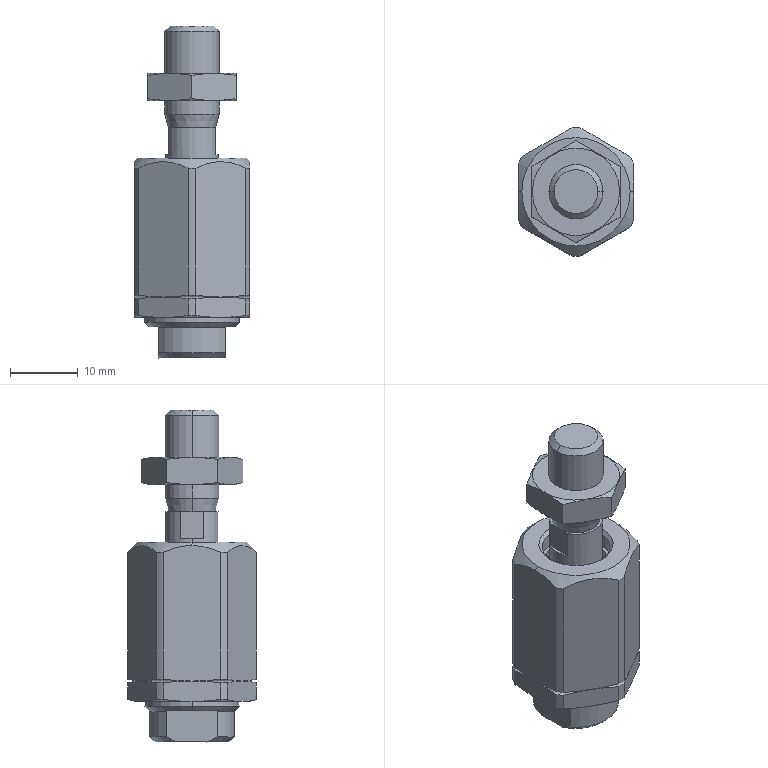Part | SolidWorks | features BaseBody 7 | 7 solids | 142 faces | box 17 x 19 x 49 mm | volume 7093 mm3 | cone 52 | plane 44 | cylinder 42 | spline 4 | commonest cylinder face diameters 19 x12 6.647 x4 9 x4 12.4 x4 12.917 x4 7.8 x2